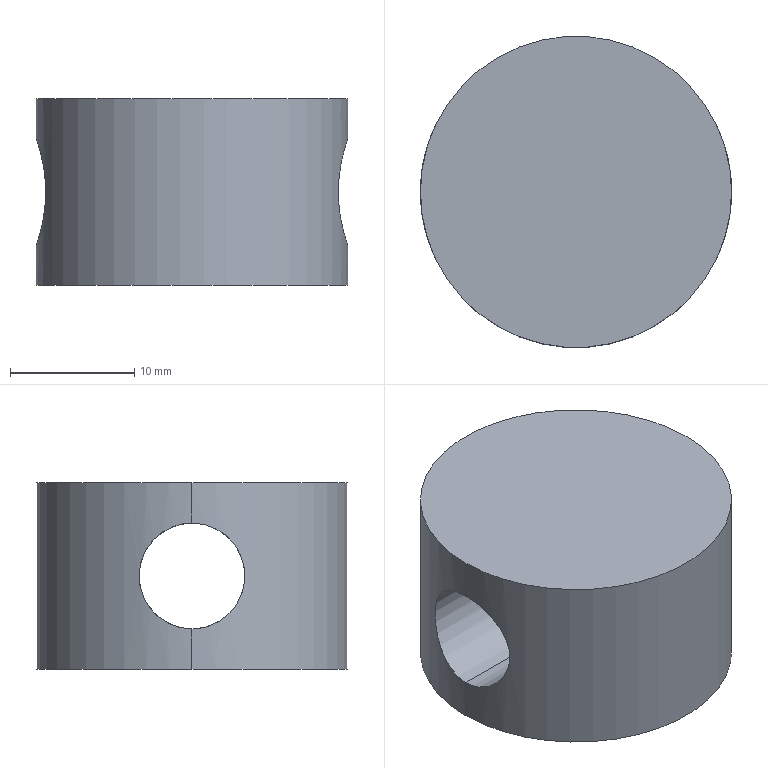Part | STEP file | Nylon shaft QY-1-30 | 1 solid | 6 faces | box 25 x 25 x 15 mm | volume 5965 mm3 | cylinder 4 | plane 2 | commonest cylinder face diameters 8.5 x2 25 x2
STEP:
#1=CARTESIAN_POINT('',(0.,0.,0.));
#2=DIRECTION('',(0.,0.,1.));
#3=DIRECTION('',(1.,0.,0.));
#4=AXIS2_PLACEMENT_3D('',#1,#2,#3);
#5=CARTESIAN_POINT('',(12.5,0.,11.75));
#6=VERTEX_POINT('',#5);
#7=CARTESIAN_POINT('',(-12.5,0.,11.75));
#8=VERTEX_POINT('',#7);
#9=CARTESIAN_POINT('',(0.,0.,11.75));
#10=DIRECTION('',(-1.,0.,0.));
#11=VECTOR('',#10,1.);
#12=LINE('',#9,#11);
#13=CARTESIAN_POINT('',(0.,0.,7.5));
#14=DIRECTION('',(-1.,0.,0.));
#15=DIRECTION('',(0.,0.,1.));
#16=AXIS2_PLACEMENT_3D('',#13,#14,#15);
#17=CYLINDRICAL_SURFACE('',#16,4.25);
#18=CARTESIAN_POINT('',(6.283,0.));
#19=DIRECTION('',(0.,1.));
#20=VECTOR('',#19,1.);
#21=LINE('',#18,#20);
#22=(GEOMETRIC_REPRESENTATION_CONTEXT(2)PARAMETRIC_REPRESENTATION_CONTEXT()REPRESENTATION_CONTEXT('',''));
#23=DEFINITIONAL_REPRESENTATION('',(#21),#22);
#24=PCURVE('',#17,#23);
#25=CARTESIAN_POINT('',(0.,0.,7.5));
#26=DIRECTION('',(-1.,0.,0.));
#27=DIRECTION('',(0.,0.,1.));
#28=AXIS2_PLACEMENT_3D('',#25,#26,#27);
#29=CYLINDRICAL_SURFACE('',#28,4.25);
#30=CARTESIAN_POINT('',(0.,0.));
#31=DIRECTION('',(0.,1.));
#32=VECTOR('',#31,1.);
#33=LINE('',#30,#32);
#34=(GEOMETRIC_REPRESENTATION_CONTEXT(2)PARAMETRIC_REPRESENTATION_CONTEXT()REPRESENTATION_CONTEXT('',''));
#35=DEFINITIONAL_REPRESENTATION('',(#33),#34);
#36=PCURVE('',#29,#35);
#37=SURFACE_CURVE('',#12,(#24,#36),.PCURVE_S1.);
#38=EDGE_CURVE('',#6,#8,#37,.T.);
#39=ORIENTED_EDGE('',*,*,#38,.T.);
#40=CARTESIAN_POINT('',(-12.5,0.,3.25));
#41=VERTEX_POINT('',#40);
#42=CARTESIAN_POINT('',(-12.5,0.,11.75));
#43=CARTESIAN_POINT('',(-12.5,-0.2788,11.75));
#44=CARTESIAN_POINT('',(-12.491,-0.5597,11.722));
#45=CARTESIAN_POINT('',(-12.454,-1.111,11.612));
#46=CARTESIAN_POINT('',(-12.427,-1.377,11.53));
#47=CARTESIAN_POINT('',(-12.359,-1.89,11.317));
#48=CARTESIAN_POINT('',(-12.318,-2.138,11.183));
#49=CARTESIAN_POINT('',(-12.229,-2.597,10.876));
#50=CARTESIAN_POINT('',(-12.182,-2.81,10.701));
#51=CARTESIAN_POINT('',(-12.036,-3.398,10.112));
#52=CARTESIAN_POINT('',(-11.939,-3.709,9.648));
#53=CARTESIAN_POINT('',(-11.833,-4.031,8.874));
#54=CARTESIAN_POINT('',(-11.804,-4.112,8.609));
#55=CARTESIAN_POINT('',(-11.766,-4.222,8.063));
#56=CARTESIAN_POINT('',(-11.755,-4.25,7.779));
#57=CARTESIAN_POINT('',(-11.755,-4.25,7.219));
#58=CARTESIAN_POINT('',(-11.765,-4.222,6.942));
#59=CARTESIAN_POINT('',(-11.804,-4.113,6.392));
#60=CARTESIAN_POINT('',(-11.833,-4.03,6.122));
#61=CARTESIAN_POINT('',(-11.904,-3.817,5.61));
#62=CARTESIAN_POINT('',(-11.946,-3.685,5.364));
#63=CARTESIAN_POINT('',(-12.037,-3.375,4.902));
#64=CARTESIAN_POINT('',(-12.085,-3.2,4.69));
#65=CARTESIAN_POINT('',(-12.182,-2.811,4.3));
#66=CARTESIAN_POINT('',(-12.23,-2.594,4.122));
#67=CARTESIAN_POINT('',(-12.319,-2.135,3.815));
#68=CARTESIAN_POINT('',(-12.359,-1.892,3.684));
#69=CARTESIAN_POINT('',(-12.427,-1.378,3.47));
#70=CARTESIAN_POINT('',(-12.454,-1.107,3.387));
#71=CARTESIAN_POINT('',(-12.49,-0.561,3.278));
#72=CARTESIAN_POINT('',(-12.5,-0.283,3.25));
#73=CARTESIAN_POINT('',(-12.5,0.,3.25));
#74=B_SPLINE_CURVE_WITH_KNOTS('',3,(#42,#43,#44,#45,#46,#47,#48,#49,#50,#51,#52,#53,#54,#55,#56,#57,#58,#59,#60,#61,#62,#63,#64,#65,#66,#67,#68,#69,#70,#71,#72,#73),.UNSPECIFIED.,.F.,.F.,(4,2,2,2,2,2,2,2,2,2,2,2,2,2,2,4),(0.01339,0.01422,0.01506,0.0159,0.01673,0.01841,0.01924,0.02008,0.02092,0.02175,0.02259,0.02343,0.02426,0.0251,0.02594,0.02677),.UNSPECIFIED.);
#75=CARTESIAN_POINT('',(6.283,12.5));
#76=CARTESIAN_POINT('',(6.267,12.5));
#77=CARTESIAN_POINT('',(6.235,12.499));
#78=CARTESIAN_POINT('',(6.187,12.494));
#79=CARTESIAN_POINT('',(6.139,12.486));
#80=CARTESIAN_POINT('',(6.091,12.474));
#81=CARTESIAN_POINT('',(6.043,12.46));
#82=CARTESIAN_POINT('',(5.996,12.442));
#83=CARTESIAN_POINT('',(5.948,12.422));
#84=CARTESIAN_POINT('',(5.901,12.399));
#85=CARTESIAN_POINT('',(5.853,12.374));
#86=CARTESIAN_POINT('',(5.805,12.347));
#87=CARTESIAN_POINT('',(5.758,12.317));
#88=CARTESIAN_POINT('',(5.71,12.286));
#89=CARTESIAN_POINT('',(5.663,12.254));
#90=CARTESIAN_POINT('',(5.616,12.22));
#91=CARTESIAN_POINT('',(5.569,12.186));
#92=CARTESIAN_POINT('',(5.521,12.151));
#93=CARTESIAN_POINT('',(5.474,12.115));
#94=CARTESIAN_POINT('',(5.426,12.08));
#95=CARTESIAN_POINT('',(5.379,12.045));
#96=CARTESIAN_POINT('',(5.332,12.011));
#97=CARTESIAN_POINT('',(5.285,11.978));
#98=CARTESIAN_POINT('',(5.237,11.947));
#99=CARTESIAN_POINT('',(5.19,11.916));
#100=CARTESIAN_POINT('',(5.142,11.888));
#101=CARTESIAN_POINT('',(5.095,11.861));
#102=CARTESIAN_POINT('',(5.047,11.837));
#103=CARTESIAN_POINT('',(4.999,11.816));
#104=CARTESIAN_POINT('',(4.952,11.798));
#105=CARTESIAN_POINT('',(4.904,11.783));
#106=CARTESIAN_POINT('',(4.857,11.771));
#107=CARTESIAN_POINT('',(4.808,11.762));
#108=CARTESIAN_POINT('',(4.76,11.757));
#109=CARTESIAN_POINT('',(4.712,11.755));
#110=CARTESIAN_POINT('',(4.664,11.757));
#111=CARTESIAN_POINT('',(4.617,11.762));
#112=CARTESIAN_POINT('',(4.569,11.77));
#113=CARTESIAN_POINT('',(4.521,11.782));
#114=CARTESIAN_POINT('',(4.473,11.798));
#115=CARTESIAN_POINT('',(4.425,11.816));
#116=CARTESIAN_POINT('',(4.377,11.838));
#117=CARTESIAN_POINT('',(4.33,11.862));
#118=CARTESIAN_POINT('',(4.282,11.888));
#119=CARTESIAN_POINT('',(4.235,11.916));
#120=CARTESIAN_POINT('',(4.187,11.947));
#121=CARTESIAN_POINT('',(4.14,11.979));
#122=CARTESIAN_POINT('',(4.092,12.012));
#123=CARTESIAN_POINT('',(4.045,12.046));
#124=CARTESIAN_POINT('',(3.998,12.081));
#125=CARTESIAN_POINT('',(3.951,12.116));
#126=CARTESIAN_POINT('',(3.904,12.151));
#127=CARTESIAN_POINT('',(3.856,12.186));
#128=CARTESIAN_POINT('',(3.809,12.221));
#129=CARTESIAN_POINT('',(3.761,12.254));
#130=CARTESIAN_POINT('',(3.714,12.287));
#131=CARTESIAN_POINT('',(3.667,12.317));
#132=CARTESIAN_POINT('',(3.619,12.347));
#133=CARTESIAN_POINT('',(3.572,12.374));
#134=CARTESIAN_POINT('',(3.525,12.399));
#135=CARTESIAN_POINT('',(3.477,12.422));
#136=CARTESIAN_POINT('',(3.429,12.442));
#137=CARTESIAN_POINT('',(3.381,12.46));
#138=CARTESIAN_POINT('',(3.333,12.474));
#139=CARTESIAN_POINT('',(3.286,12.486));
#140=CARTESIAN_POINT('',(3.238,12.494));
#141=CARTESIAN_POINT('',(3.19,12.499));
#142=CARTESIAN_POINT('',(3.158,12.5));
#143=CARTESIAN_POINT('',(3.142,12.5));
#144=B_SPLINE_CURVE_WITH_KNOTS('',3,(#75,#76,#77,#78,#79,#80,#81,#82,#83,#84,#85,#86,#87,#88,#89,#90,#91,#92,#93,#94,#95,#96,#97,#98,#99,#100,#101,#102,#103,#104,#105,#106,#107,#108,#109,#110,#111,#112,#113,#114,#115,#116,#117,#118,#119,#120,#121,#122,#123,#124,#125,#126,#127,#128,#129,#130,#131,#132,#133,#134,#135,#136,#137,#138,#139,#140,#141,#142,#143),.UNSPECIFIED.,.F.,.F.,(4,1,1,1,1,1,1,1,1,1,1,1,1,1,1,1,1,1,1,1,1,1,1,1,1,1,1,1,1,1,1,1,1,1,1,1,1,1,1,1,1,1,1,1,1,1,1,1,1,1,1,1,1,1,1,1,1,1,1,1,1,1,1,1,1,1,4),(0.01339,0.01359,0.01379,0.014,0.0142,0.0144,0.0146,0.01481,0.01501,0.01521,0.01542,0.01562,0.01582,0.01602,0.01623,0.01643,0.01663,0.01684,0.01704,0.01724,0.01744,0.01765,0.01785,0.01805,0.01826,0.01846,0.01866,0.01886,0.01907,0.01927,0.01947,0.01967,0.01988,0.02008,0.02028,0.02049,0.02069,0.02089,0.02109,0.0213,0.0215,0.0217,0.02191,0.02211,0.02231,0.02251,0.02272,0.02292,0.02312,0.02333,0.02353,0.02373,0.02393,0.02414,0.02434,0.02454,0.02474,0.02495,0.02515,0.02535,0.02556,0.02576,0.02596,0.02616,0.02637,0.02657,0.02677),.QUASI_UNIFORM_KNOTS.);
#145=(GEOMETRIC_REPRESENTATION_CONTEXT(2)PARAMETRIC_REPRESENTATION_CONTEXT()REPRESENTATION_CONTEXT('',''));
#146=DEFINITIONAL_REPRESENTATION('',(#144),#145);
#147=PCURVE('',#17,#146);
#148=CARTESIAN_POINT('',(0.,0.,15.));
#149=DIRECTION('',(0.,0.,-1.));
#150=DIRECTION('',(-1.,0.,0.));
#151=AXIS2_PLACEMENT_3D('',#148,#149,#150);
#152=CYLINDRICAL_SURFACE('',#151,12.5);
#153=CARTESIAN_POINT('',(6.283,3.25));
#154=CARTESIAN_POINT('',(6.278,3.25));
#155=CARTESIAN_POINT('',(6.267,3.253));
#156=CARTESIAN_POINT('',(6.251,3.268));
#157=CARTESIAN_POINT('',(6.234,3.292));
#158=CARTESIAN_POINT('',(6.218,3.326));
#159=CARTESIAN_POINT('',(6.202,3.37));
#160=CARTESIAN_POINT('',(6.187,3.423));
#161=CARTESIAN_POINT('',(6.171,3.485));
#162=CARTESIAN_POINT('',(6.156,3.556));
#163=CARTESIAN_POINT('',(6.141,3.636));
#164=CARTESIAN_POINT('',(6.126,3.725));
#165=CARTESIAN_POINT('',(6.112,3.822));
#166=CARTESIAN_POINT('',(6.098,3.928));
#167=CARTESIAN_POINT('',(6.084,4.041));
#168=CARTESIAN_POINT('',(6.071,4.161));
#169=CARTESIAN_POINT('',(6.058,4.289));
#170=CARTESIAN_POINT('',(6.046,4.424));
#171=CARTESIAN_POINT('',(6.034,4.567));
#172=CARTESIAN_POINT('',(6.023,4.716));
#173=CARTESIAN_POINT('',(6.013,4.871));
#174=CARTESIAN_POINT('',(6.003,5.031));
#175=CARTESIAN_POINT('',(5.993,5.197));
#176=CARTESIAN_POINT('',(5.984,5.369));
#177=CARTESIAN_POINT('',(5.976,5.546));
#178=CARTESIAN_POINT('',(5.969,5.727));
#179=CARTESIAN_POINT('',(5.962,5.914));
#180=CARTESIAN_POINT('',(5.956,6.104));
#181=CARTESIAN_POINT('',(5.951,6.296));
#182=CARTESIAN_POINT('',(5.946,6.491));
#183=CARTESIAN_POINT('',(5.943,6.688));
#184=CARTESIAN_POINT('',(5.94,6.889));
#185=CARTESIAN_POINT('',(5.938,7.092));
#186=CARTESIAN_POINT('',(5.937,7.297));
#187=CARTESIAN_POINT('',(5.936,7.501));
#188=CARTESIAN_POINT('',(5.937,7.704));
#189=CARTESIAN_POINT('',(5.938,7.906));
#190=CARTESIAN_POINT('',(5.94,8.108));
#191=CARTESIAN_POINT('',(5.943,8.308));
#192=CARTESIAN_POINT('',(5.946,8.507));
#193=CARTESIAN_POINT('',(5.951,8.704));
#194=CARTESIAN_POINT('',(5.956,8.898));
#195=CARTESIAN_POINT('',(5.962,9.088));
#196=CARTESIAN_POINT('',(5.969,9.273));
#197=CARTESIAN_POINT('',(5.976,9.454));
#198=CARTESIAN_POINT('',(5.984,9.632));
#199=CARTESIAN_POINT('',(5.993,9.804));
#200=CARTESIAN_POINT('',(6.003,9.971));
#201=CARTESIAN_POINT('',(6.013,10.132));
#202=CARTESIAN_POINT('',(6.023,10.286));
#203=CARTESIAN_POINT('',(6.035,10.434));
#204=CARTESIAN_POINT('',(6.046,10.576));
#205=CARTESIAN_POINT('',(6.058,10.712));
#206=CARTESIAN_POINT('',(6.071,10.84));
#207=CARTESIAN_POINT('',(6.084,10.962));
#208=CARTESIAN_POINT('',(6.098,11.074));
#209=CARTESIAN_POINT('',(6.112,11.179));
#210=CARTESIAN_POINT('',(6.126,11.275));
#211=CARTESIAN_POINT('',(6.141,11.364));
#212=CARTESIAN_POINT('',(6.156,11.444));
#213=CARTESIAN_POINT('',(6.171,11.515));
#214=CARTESIAN_POINT('',(6.187,11.577));
#215=CARTESIAN_POINT('',(6.203,11.631));
#216=CARTESIAN_POINT('',(6.218,11.674));
#217=CARTESIAN_POINT('',(6.234,11.708));
#218=CARTESIAN_POINT('',(6.251,11.732));
#219=CARTESIAN_POINT('',(6.267,11.747));
#220=CARTESIAN_POINT('',(6.278,11.75));
#221=CARTESIAN_POINT('',(6.283,11.75));
#222=B_SPLINE_CURVE_WITH_KNOTS('',3,(#153,#154,#155,#156,#157,#158,#159,#160,#161,#162,#163,#164,#165,#166,#167,#168,#169,#170,#171,#172,#173,#174,#175,#176,#177,#178,#179,#180,#181,#182,#183,#184,#185,#186,#187,#188,#189,#190,#191,#192,#193,#194,#195,#196,#197,#198,#199,#200,#201,#202,#203,#204,#205,#206,#207,#208,#209,#210,#211,#212,#213,#214,#215,#216,#217,#218,#219,#220,#221),.UNSPECIFIED.,.F.,.F.,(4,1,1,1,1,1,1,1,1,1,1,1,1,1,1,1,1,1,1,1,1,1,1,1,1,1,1,1,1,1,1,1,1,1,1,1,1,1,1,1,1,1,1,1,1,1,1,1,1,1,1,1,1,1,1,1,1,1,1,1,1,1,1,1,1,1,4),(0.01339,0.01359,0.01379,0.014,0.0142,0.0144,0.0146,0.01481,0.01501,0.01521,0.01542,0.01562,0.01582,0.01602,0.01623,0.01643,0.01663,0.01684,0.01704,0.01724,0.01744,0.01765,0.01785,0.01805,0.01826,0.01846,0.01866,0.01886,0.01907,0.01927,0.01947,0.01967,0.01988,0.02008,0.02028,0.02049,0.02069,0.02089,0.02109,0.0213,0.0215,0.0217,0.02191,0.02211,0.02231,0.02251,0.02272,0.02292,0.02312,0.02333,0.02353,0.02373,0.02393,0.02414,0.02434,0.02454,0.02474,0.02495,0.02515,0.02535,0.02556,0.02576,0.02596,0.02616,0.02637,0.02657,0.02677),.QUASI_UNIFORM_KNOTS.);
#223=(GEOMETRIC_REPRESENTATION_CONTEXT(2)PARAMETRIC_REPRESENTATION_CONTEXT()REPRESENTATION_CONTEXT('',''));
#224=DEFINITIONAL_REPRESENTATION('',(#222),#223);
#225=PCURVE('',#152,#224);
#226=SURFACE_CURVE('',#74,(#147,#225),.PCURVE_S1.);
#227=EDGE_CURVE('',#8,#41,#226,.T.);
#228=ORIENTED_EDGE('',*,*,#227,.T.);
#229=CARTESIAN_POINT('',(12.5,0.,3.25));
#230=VERTEX_POINT('',#229);
#231=CARTESIAN_POINT('',(0.,0.,3.25));
#232=DIRECTION('',(-1.,0.,0.));
#233=VECTOR('',#232,1.);
#234=LINE('',#231,#233);
#235=CARTESIAN_POINT('',(3.142,0.));
#236=DIRECTION('',(0.,1.));
#237=VECTOR('',#236,1.);
#238=LINE('',#235,#237);
#239=(GEOMETRIC_REPRESENTATION_CONTEXT(2)PARAMETRIC_REPRESENTATION_CONTEXT()REPRESENTATION_CONTEXT('',''));
#240=DEFINITIONAL_REPRESENTATION('',(#238),#239);
#241=PCURVE('',#17,#240);
#242=CARTESIAN_POINT('',(3.142,0.));
#243=DIRECTION('',(0.,1.));
#244=VECTOR('',#243,1.);
#245=LINE('',#242,#244);
#246=(GEOMETRIC_REPRESENTATION_CONTEXT(2)PARAMETRIC_REPRESENTATION_CONTEXT()REPRESENTATION_CONTEXT('',''));
#247=DEFINITIONAL_REPRESENTATION('',(#245),#246);
#248=PCURVE('',#29,#247);
#249=SURFACE_CURVE('',#234,(#241,#248),.PCURVE_S1.);
#250=EDGE_CURVE('',#230,#41,#249,.T.);
#251=ORIENTED_EDGE('',*,*,#250,.F.);
#252=CARTESIAN_POINT('',(12.5,0.,3.25));
#253=CARTESIAN_POINT('',(12.5,-0.2788,3.25));
#254=CARTESIAN_POINT('',(12.491,-0.5597,3.278));
#255=CARTESIAN_POINT('',(12.454,-1.111,3.388));
#256=CARTESIAN_POINT('',(12.427,-1.377,3.47));
#257=CARTESIAN_POINT('',(12.359,-1.89,3.683));
#258=CARTESIAN_POINT('',(12.318,-2.138,3.817));
#259=CARTESIAN_POINT('',(12.229,-2.597,4.124));
#260=CARTESIAN_POINT('',(12.182,-2.81,4.299));
#261=CARTESIAN_POINT('',(12.036,-3.398,4.888));
#262=CARTESIAN_POINT('',(11.939,-3.709,5.352));
#263=CARTESIAN_POINT('',(11.833,-4.031,6.126));
#264=CARTESIAN_POINT('',(11.804,-4.112,6.391));
#265=CARTESIAN_POINT('',(11.766,-4.222,6.937));
#266=CARTESIAN_POINT('',(11.755,-4.25,7.221));
#267=CARTESIAN_POINT('',(11.755,-4.25,7.781));
#268=CARTESIAN_POINT('',(11.765,-4.222,8.058));
#269=CARTESIAN_POINT('',(11.804,-4.113,8.608));
#270=CARTESIAN_POINT('',(11.833,-4.03,8.878));
#271=CARTESIAN_POINT('',(11.904,-3.817,9.39));
#272=CARTESIAN_POINT('',(11.946,-3.685,9.636));
#273=CARTESIAN_POINT('',(12.037,-3.375,10.098));
#274=CARTESIAN_POINT('',(12.085,-3.2,10.31));
#275=CARTESIAN_POINT('',(12.182,-2.811,10.7));
#276=CARTESIAN_POINT('',(12.23,-2.594,10.878));
#277=CARTESIAN_POINT('',(12.319,-2.135,11.185));
#278=CARTESIAN_POINT('',(12.359,-1.892,11.316));
#279=CARTESIAN_POINT('',(12.427,-1.378,11.53));
#280=CARTESIAN_POINT('',(12.454,-1.107,11.613));
#281=CARTESIAN_POINT('',(12.49,-0.561,11.722));
#282=CARTESIAN_POINT('',(12.5,-0.283,11.75));
#283=CARTESIAN_POINT('',(12.5,0.,11.75));
#284=B_SPLINE_CURVE_WITH_KNOTS('',3,(#252,#253,#254,#255,#256,#257,#258,#259,#260,#261,#262,#263,#264,#265,#266,#267,#268,#269,#270,#271,#272,#273,#274,#275,#276,#277,#278,#279,#280,#281,#282,#283),.UNSPECIFIED.,.F.,.F.,(4,2,2,2,2,2,2,2,2,2,2,2,2,2,2,4),(0.01339,0.01422,0.01506,0.0159,0.01673,0.01841,0.01924,0.02008,0.02092,0.02175,0.02259,0.02343,0.02426,0.0251,0.02594,0.02677),.UNSPECIFIED.);
#285=CARTESIAN_POINT('',(3.142,-12.5));
#286=CARTESIAN_POINT('',(3.157,-12.5));
#287=CARTESIAN_POINT('',(3.189,-12.499));
#288=CARTESIAN_POINT('',(3.237,-12.494));
#289=CARTESIAN_POINT('',(3.285,-12.486));
#290=CARTESIAN_POINT('',(3.333,-12.474));
#291=CARTESIAN_POINT('',(3.381,-12.46));
#292=CARTESIAN_POINT('',(3.429,-12.442));
#293=CARTESIAN_POINT('',(3.477,-12.422));
#294=CARTESIAN_POINT('',(3.524,-12.399));
#295=CARTESIAN_POINT('',(3.572,-12.374));
#296=CARTESIAN_POINT('',(3.619,-12.347));
#297=CARTESIAN_POINT('',(3.667,-12.317));
#298=CARTESIAN_POINT('',(3.715,-12.286));
#299=CARTESIAN_POINT('',(3.762,-12.254));
#300=CARTESIAN_POINT('',(3.809,-12.22));
#301=CARTESIAN_POINT('',(3.856,-12.186));
#302=CARTESIAN_POINT('',(3.903,-12.151));
#303=CARTESIAN_POINT('',(3.951,-12.115));
#304=CARTESIAN_POINT('',(3.998,-12.08));
#305=CARTESIAN_POINT('',(4.046,-12.045));
#306=CARTESIAN_POINT('',(4.093,-12.011));
#307=CARTESIAN_POINT('',(4.14,-11.978));
#308=CARTESIAN_POINT('',(4.187,-11.947));
#309=CARTESIAN_POINT('',(4.235,-11.916));
#310=CARTESIAN_POINT('',(4.282,-11.888));
#311=CARTESIAN_POINT('',(4.33,-11.861));
#312=CARTESIAN_POINT('',(4.378,-11.837));
#313=CARTESIAN_POINT('',(4.425,-11.816));
#314=CARTESIAN_POINT('',(4.473,-11.798));
#315=CARTESIAN_POINT('',(4.52,-11.783));
#316=CARTESIAN_POINT('',(4.568,-11.771));
#317=CARTESIAN_POINT('',(4.616,-11.762));
#318=CARTESIAN_POINT('',(4.665,-11.757));
#319=CARTESIAN_POINT('',(4.713,-11.755));
#320=CARTESIAN_POINT('',(4.76,-11.757));
#321=CARTESIAN_POINT('',(4.808,-11.762));
#322=CARTESIAN_POINT('',(4.856,-11.77));
#323=CARTESIAN_POINT('',(4.904,-11.782));
#324=CARTESIAN_POINT('',(4.952,-11.798));
#325=CARTESIAN_POINT('',(5.,-11.816));
#326=CARTESIAN_POINT('',(5.047,-11.838));
#327=CARTESIAN_POINT('',(5.095,-11.862));
#328=CARTESIAN_POINT('',(5.143,-11.888));
#329=CARTESIAN_POINT('',(5.19,-11.916));
#330=CARTESIAN_POINT('',(5.238,-11.947));
#331=CARTESIAN_POINT('',(5.285,-11.979));
#332=CARTESIAN_POINT('',(5.333,-12.012));
#333=CARTESIAN_POINT('',(5.38,-12.046));
#334=CARTESIAN_POINT('',(5.427,-12.081));
#335=CARTESIAN_POINT('',(5.474,-12.116));
#336=CARTESIAN_POINT('',(5.521,-12.151));
#337=CARTESIAN_POINT('',(5.569,-12.186));
#338=CARTESIAN_POINT('',(5.616,-12.221));
#339=CARTESIAN_POINT('',(5.664,-12.254));
#340=CARTESIAN_POINT('',(5.711,-12.287));
#341=CARTESIAN_POINT('',(5.758,-12.317));
#342=CARTESIAN_POINT('',(5.805,-12.347));
#343=CARTESIAN_POINT('',(5.853,-12.374));
#344=CARTESIAN_POINT('',(5.9,-12.399));
#345=CARTESIAN_POINT('',(5.948,-12.422));
#346=CARTESIAN_POINT('',(5.996,-12.442));
#347=CARTESIAN_POINT('',(6.044,-12.46));
#348=CARTESIAN_POINT('',(6.092,-12.474));
#349=CARTESIAN_POINT('',(6.139,-12.486));
#350=CARTESIAN_POINT('',(6.187,-12.494));
#351=CARTESIAN_POINT('',(6.235,-12.499));
#352=CARTESIAN_POINT('',(6.267,-12.5));
#353=CARTESIAN_POINT('',(6.283,-12.5));
#354=B_SPLINE_CURVE_WITH_KNOTS('',3,(#285,#286,#287,#288,#289,#290,#291,#292,#293,#294,#295,#296,#297,#298,#299,#300,#301,#302,#303,#304,#305,#306,#307,#308,#309,#310,#311,#312,#313,#314,#315,#316,#317,#318,#319,#320,#321,#322,#323,#324,#325,#326,#327,#328,#329,#330,#331,#332,#333,#334,#335,#336,#337,#338,#339,#340,#341,#342,#343,#344,#345,#346,#347,#348,#349,#350,#351,#352,#353),.UNSPECIFIED.,.F.,.F.,(4,1,1,1,1,1,1,1,1,1,1,1,1,1,1,1,1,1,1,1,1,1,1,1,1,1,1,1,1,1,1,1,1,1,1,1,1,1,1,1,1,1,1,1,1,1,1,1,1,1,1,1,1,1,1,1,1,1,1,1,1,1,1,1,1,1,4),(0.01339,0.01359,0.01379,0.014,0.0142,0.0144,0.0146,0.01481,0.01501,0.01521,0.01542,0.01562,0.01582,0.01602,0.01623,0.01643,0.01663,0.01684,0.01704,0.01724,0.01744,0.01765,0.01785,0.01805,0.01826,0.01846,0.01866,0.01886,0.01907,0.01927,0.01947,0.01967,0.01988,0.02008,0.02028,0.02049,0.02069,0.02089,0.02109,0.0213,0.0215,0.0217,0.02191,0.02211,0.02231,0.02251,0.02272,0.02292,0.02312,0.02333,0.02353,0.02373,0.02393,0.02414,0.02434,0.02454,0.02474,0.02495,0.02515,0.02535,0.02556,0.02576,0.02596,0.02616,0.02637,0.02657,0.02677),.QUASI_UNIFORM_KNOTS.);
#355=(GEOMETRIC_REPRESENTATION_CONTEXT(2)PARAMETRIC_REPRESENTATION_CONTEXT()REPRESENTATION_CONTEXT('',''));
#356=DEFINITIONAL_REPRESENTATION('',(#354),#355);
#357=PCURVE('',#17,#356);
#358=CARTESIAN_POINT('',(3.142,11.75));
#359=CARTESIAN_POINT('',(3.147,11.75));
#360=CARTESIAN_POINT('',(3.158,11.747));
#361=CARTESIAN_POINT('',(3.174,11.732));
#362=CARTESIAN_POINT('',(3.19,11.708));
#363=CARTESIAN_POINT('',(3.206,11.674));
#364=CARTESIAN_POINT('',(3.222,11.63));
#365=CARTESIAN_POINT('',(3.238,11.577));
#366=CARTESIAN_POINT('',(3.254,11.515));
#367=CARTESIAN_POINT('',(3.269,11.444));
#368=CARTESIAN_POINT('',(3.284,11.364));
#369=CARTESIAN_POINT('',(3.299,11.275));
#370=CARTESIAN_POINT('',(3.313,11.178));
#371=CARTESIAN_POINT('',(3.327,11.072));
#372=CARTESIAN_POINT('',(3.341,10.959));
#373=CARTESIAN_POINT('',(3.354,10.839));
#374=CARTESIAN_POINT('',(3.366,10.711));
#375=CARTESIAN_POINT('',(3.379,10.576));
#376=CARTESIAN_POINT('',(3.39,10.433));
#377=CARTESIAN_POINT('',(3.402,10.284));
#378=CARTESIAN_POINT('',(3.412,10.129));
#379=CARTESIAN_POINT('',(3.422,9.969));
#380=CARTESIAN_POINT('',(3.432,9.803));
#381=CARTESIAN_POINT('',(3.44,9.631));
#382=CARTESIAN_POINT('',(3.448,9.454));
#383=CARTESIAN_POINT('',(3.456,9.273));
#384=CARTESIAN_POINT('',(3.463,9.086));
#385=CARTESIAN_POINT('',(3.469,8.896));
#386=CARTESIAN_POINT('',(3.474,8.704));
#387=CARTESIAN_POINT('',(3.478,8.509));
#388=CARTESIAN_POINT('',(3.482,8.312));
#389=CARTESIAN_POINT('',(3.485,8.111));
#390=CARTESIAN_POINT('',(3.487,7.908));
#391=CARTESIAN_POINT('',(3.488,7.703));
#392=CARTESIAN_POINT('',(3.489,7.499));
#393=CARTESIAN_POINT('',(3.488,7.296));
#394=CARTESIAN_POINT('',(3.487,7.094));
#395=CARTESIAN_POINT('',(3.485,6.892));
#396=CARTESIAN_POINT('',(3.482,6.692));
#397=CARTESIAN_POINT('',(3.478,6.493));
#398=CARTESIAN_POINT('',(3.474,6.296));
#399=CARTESIAN_POINT('',(3.469,6.102));
#400=CARTESIAN_POINT('',(3.463,5.912));
#401=CARTESIAN_POINT('',(3.456,5.727));
#402=CARTESIAN_POINT('',(3.448,5.546));
#403=CARTESIAN_POINT('',(3.44,5.368));
#404=CARTESIAN_POINT('',(3.431,5.196));
#405=CARTESIAN_POINT('',(3.422,5.029));
#406=CARTESIAN_POINT('',(3.412,4.868));
#407=CARTESIAN_POINT('',(3.401,4.714));
#408=CARTESIAN_POINT('',(3.39,4.566));
#409=CARTESIAN_POINT('',(3.379,4.424));
#410=CARTESIAN_POINT('',(3.366,4.288));
#411=CARTESIAN_POINT('',(3.354,4.16));
#412=CARTESIAN_POINT('',(3.34,4.038));
#413=CARTESIAN_POINT('',(3.327,3.926));
#414=CARTESIAN_POINT('',(3.313,3.821));
#415=CARTESIAN_POINT('',(3.299,3.725));
#416=CARTESIAN_POINT('',(3.284,3.636));
#417=CARTESIAN_POINT('',(3.269,3.556));
#418=CARTESIAN_POINT('',(3.254,3.485));
#419=CARTESIAN_POINT('',(3.238,3.423));
#420=CARTESIAN_POINT('',(3.222,3.369));
#421=CARTESIAN_POINT('',(3.206,3.326));
#422=CARTESIAN_POINT('',(3.19,3.292));
#423=CARTESIAN_POINT('',(3.174,3.268));
#424=CARTESIAN_POINT('',(3.158,3.253));
#425=CARTESIAN_POINT('',(3.147,3.25));
#426=CARTESIAN_POINT('',(3.142,3.25));
#427=B_SPLINE_CURVE_WITH_KNOTS('',3,(#358,#359,#360,#361,#362,#363,#364,#365,#366,#367,#368,#369,#370,#371,#372,#373,#374,#375,#376,#377,#378,#379,#380,#381,#382,#383,#384,#385,#386,#387,#388,#389,#390,#391,#392,#393,#394,#395,#396,#397,#398,#399,#400,#401,#402,#403,#404,#405,#406,#407,#408,#409,#410,#411,#412,#413,#414,#415,#416,#417,#418,#419,#420,#421,#422,#423,#424,#425,#426),.UNSPECIFIED.,.F.,.F.,(4,1,1,1,1,1,1,1,1,1,1,1,1,1,1,1,1,1,1,1,1,1,1,1,1,1,1,1,1,1,1,1,1,1,1,1,1,1,1,1,1,1,1,1,1,1,1,1,1,1,1,1,1,1,1,1,1,1,1,1,1,1,1,1,1,1,4),(0.01339,0.01359,0.01379,0.014,0.0142,0.0144,0.0146,0.01481,0.01501,0.01521,0.01542,0.01562,0.01582,0.01602,0.01623,0.01643,0.01663,0.01684,0.01704,0.01724,0.01744,0.01765,0.01785,0.01805,0.01826,0.01846,0.01866,0.01886,0.01907,0.01927,0.01947,0.01967,0.01988,0.02008,0.02028,0.02049,0.02069,0.02089,0.02109,0.0213,0.0215,0.0217,0.02191,0.02211,0.02231,0.02251,0.02272,0.02292,0.02312,0.02333,0.02353,0.02373,0.02393,0.02414,0.02434,0.02454,0.02474,0.02495,0.02515,0.02535,0.02556,0.02576,0.02596,0.02616,0.02637,0.02657,0.02677),.QUASI_UNIFORM_KNOTS.);
#428=(GEOMETRIC_REPRESENTATION_CONTEXT(2)PARAMETRIC_REPRESENTATION_CONTEXT()REPRESENTATION_CONTEXT('',''));
#429=DEFINITIONAL_REPRESENTATION('',(#427),#428);
#430=PCURVE('',#152,#429);
#431=SURFACE_CURVE('',#284,(#357,#430),.PCURVE_S1.);
#432=EDGE_CURVE('',#230,#6,#431,.T.);
#433=ORIENTED_EDGE('',*,*,#432,.T.);
#434=EDGE_LOOP('',(#39,#228,#251,#433));
#435=FACE_BOUND('',#434,.F.);
#436=ADVANCED_FACE('',(#435),#17,.F.);
#437=CARTESIAN_POINT('',(12.5,0.,15.));
#438=VERTEX_POINT('',#437);
#439=CARTESIAN_POINT('',(-12.5,0.,15.));
#440=VERTEX_POINT('',#439);
#441=CARTESIAN_POINT('',(0.,0.,15.));
#442=DIRECTION('',(0.,0.,1.));
#443=DIRECTION('',(1.,0.,0.));
#444=AXIS2_PLACEMENT_3D('',#441,#442,#443);
#445=CIRCLE('',#444,12.5);
#446=CARTESIAN_POINT('',(0.,0.,15.));
#447=DIRECTION('',(0.,0.,-1.));
#448=DIRECTION('',(-1.,0.,0.));
#449=AXIS2_PLACEMENT_3D('',#446,#447,#448);
#450=CYLINDRICAL_SURFACE('',#449,12.5);
#451=CARTESIAN_POINT('',(3.142,0.));
#452=DIRECTION('',(-1.,0.));
#453=VECTOR('',#452,1.);
#454=LINE('',#451,#453);
#455=(GEOMETRIC_REPRESENTATION_CONTEXT(2)PARAMETRIC_REPRESENTATION_CONTEXT()REPRESENTATION_CONTEXT('',''));
#456=DEFINITIONAL_REPRESENTATION('',(#454),#455);
#457=PCURVE('',#450,#456);
#458=CARTESIAN_POINT('',(0.,0.,15.));
#459=DIRECTION('',(0.,0.,1.));
#460=DIRECTION('',(1.,0.,0.));
#461=AXIS2_PLACEMENT_3D('',#458,#459,#460);
#462=PLANE('',#461);
#463=CARTESIAN_POINT('',(0.,0.));
#464=DIRECTION('',(1.,0.));
#465=AXIS2_PLACEMENT_2D('',#463,#464);
#466=CIRCLE('',#465,12.5);
#467=(GEOMETRIC_REPRESENTATION_CONTEXT(2)PARAMETRIC_REPRESENTATION_CONTEXT()REPRESENTATION_CONTEXT('',''));
#468=DEFINITIONAL_REPRESENTATION('',(#466),#467);
#469=PCURVE('',#462,#468);
#470=SURFACE_CURVE('',#445,(#457,#469),.PCURVE_S1.);
#471=EDGE_CURVE('',#438,#440,#470,.T.);
#472=ORIENTED_EDGE('',*,*,#471,.F.);
#473=CARTESIAN_POINT('',(12.5,0.,15.));
#474=DIRECTION('',(0.,0.,-1.));
#475=VECTOR('',#474,1.);
#476=LINE('',#473,#475);
#477=CARTESIAN_POINT('',(3.142,0.));
#478=DIRECTION('',(0.,1.));
#479=VECTOR('',#478,1.);
#480=LINE('',#477,#479);
#481=(GEOMETRIC_REPRESENTATION_CONTEXT(2)PARAMETRIC_REPRESENTATION_CONTEXT()REPRESENTATION_CONTEXT('',''));
#482=DEFINITIONAL_REPRESENTATION('',(#480),#481);
#483=PCURVE('',#450,#482);
#484=CARTESIAN_POINT('',(3.142,0.));
#485=DIRECTION('',(0.,1.));
#486=VECTOR('',#485,1.);
#487=LINE('',#484,#486);
#488=(GEOMETRIC_REPRESENTATION_CONTEXT(2)PARAMETRIC_REPRESENTATION_CONTEXT()REPRESENTATION_CONTEXT('',''));
#489=DEFINITIONAL_REPRESENTATION('',(#487),#488);
#490=PCURVE('',#152,#489);
#491=SURFACE_CURVE('',#476,(#483,#490),.PCURVE_S1.);
#492=EDGE_CURVE('',#438,#6,#491,.T.);
#493=ORIENTED_EDGE('',*,*,#492,.T.);
#494=CARTESIAN_POINT('',(12.5,0.,11.75));
#495=CARTESIAN_POINT('',(12.5,0.2831,11.75));
#496=CARTESIAN_POINT('',(12.49,0.561,11.722));
#497=CARTESIAN_POINT('',(12.454,1.107,11.613));
#498=CARTESIAN_POINT('',(12.426,1.378,11.53));
#499=CARTESIAN_POINT('',(12.359,1.892,11.316));
#500=CARTESIAN_POINT('',(12.318,2.136,11.185));
#501=CARTESIAN_POINT('',(12.23,2.596,10.876));
#502=CARTESIAN_POINT('',(12.181,2.812,10.698));
#503=CARTESIAN_POINT('',(12.085,3.201,10.309));
#504=CARTESIAN_POINT('',(12.037,3.376,10.097));
#505=CARTESIAN_POINT('',(11.945,3.687,9.633));
#506=CARTESIAN_POINT('',(11.903,3.817,9.389));
#507=CARTESIAN_POINT('',(11.833,4.03,8.879));
#508=CARTESIAN_POINT('',(11.804,4.112,8.609));
#509=CARTESIAN_POINT('',(11.765,4.222,8.059));
#510=CARTESIAN_POINT('',(11.755,4.25,7.782));
#511=CARTESIAN_POINT('',(11.755,4.25,7.223));
#512=CARTESIAN_POINT('',(11.766,4.222,6.939));
#513=CARTESIAN_POINT('',(11.804,4.112,6.392));
#514=CARTESIAN_POINT('',(11.833,4.031,6.126));
#515=CARTESIAN_POINT('',(11.904,3.816,5.608));
#516=CARTESIAN_POINT('',(11.946,3.684,5.364));
#517=CARTESIAN_POINT('',(12.036,3.377,4.905));
#518=CARTESIAN_POINT('',(12.085,3.2,4.689));
#519=CARTESIAN_POINT('',(12.182,2.808,4.298));
#520=CARTESIAN_POINT('',(12.23,2.596,4.124));
#521=CARTESIAN_POINT('',(12.318,2.137,3.816));
#522=CARTESIAN_POINT('',(12.359,1.888,3.682));
#523=CARTESIAN_POINT('',(12.427,1.376,3.47));
#524=CARTESIAN_POINT('',(12.454,1.111,3.388));
#525=CARTESIAN_POINT('',(12.49,0.5605,3.278));
#526=CARTESIAN_POINT('',(12.5,0.2789,3.25));
#527=CARTESIAN_POINT('',(12.5,0.,3.25));
#528=B_SPLINE_CURVE_WITH_KNOTS('',3,(#494,#495,#496,#497,#498,#499,#500,#501,#502,#503,#504,#505,#506,#507,#508,#509,#510,#511,#512,#513,#514,#515,#516,#517,#518,#519,#520,#521,#522,#523,#524,#525,#526,#527),.UNSPECIFIED.,.F.,.F.,(4,2,2,2,2,2,2,2,2,2,2,2,2,2,2,2,4),(0.,0.0008368,0.001674,0.00251,0.003347,0.004184,0.005021,0.005857,0.006694,0.007531,0.008368,0.009204,0.01004,0.01088,0.01171,0.01255,0.01339),.UNSPECIFIED.);
#529=CARTESIAN_POINT('',(3.142,3.25));
#530=CARTESIAN_POINT('',(3.136,3.25));
#531=CARTESIAN_POINT('',(3.125,3.253));
#532=CARTESIAN_POINT('',(3.109,3.268));
#533=CARTESIAN_POINT('',(3.093,3.292));
#534=CARTESIAN_POINT('',(3.077,3.326));
#535=CARTESIAN_POINT('',(3.061,3.37));
#536=CARTESIAN_POINT('',(3.045,3.423));
#537=CARTESIAN_POINT('',(3.029,3.485));
#538=CARTESIAN_POINT('',(3.014,3.557));
#539=CARTESIAN_POINT('',(2.999,3.637));
#540=CARTESIAN_POINT('',(2.984,3.725));
#541=CARTESIAN_POINT('',(2.97,3.822));
#542=CARTESIAN_POINT('',(2.956,3.926));
#543=CARTESIAN_POINT('',(2.943,4.04));
#544=CARTESIAN_POINT('',(2.929,4.161));
#545=CARTESIAN_POINT('',(2.917,4.29));
#546=CARTESIAN_POINT('',(2.904,4.425));
#547=CARTESIAN_POINT('',(2.893,4.567));
#548=CARTESIAN_POINT('',(2.882,4.715));
#549=CARTESIAN_POINT('',(2.871,4.869));
#550=CARTESIAN_POINT('',(2.861,5.03));
#551=CARTESIAN_POINT('',(2.852,5.198));
#552=CARTESIAN_POINT('',(2.843,5.37));
#553=CARTESIAN_POINT('',(2.835,5.547));
#554=CARTESIAN_POINT('',(2.827,5.727));
#555=CARTESIAN_POINT('',(2.821,5.912));
#556=CARTESIAN_POINT('',(2.815,6.101));
#557=CARTESIAN_POINT('',(2.809,6.295));
#558=CARTESIAN_POINT('',(2.805,6.492));
#559=CARTESIAN_POINT('',(2.801,6.691));
#560=CARTESIAN_POINT('',(2.798,6.892));
#561=CARTESIAN_POINT('',(2.796,7.093));
#562=CARTESIAN_POINT('',(2.795,7.295));
#563=CARTESIAN_POINT('',(2.795,7.498));
#564=CARTESIAN_POINT('',(2.795,7.702));
#565=CARTESIAN_POINT('',(2.796,7.906));
#566=CARTESIAN_POINT('',(2.798,8.11));
#567=CARTESIAN_POINT('',(2.801,8.311));
#568=CARTESIAN_POINT('',(2.805,8.508));
#569=CARTESIAN_POINT('',(2.809,8.704));
#570=CARTESIAN_POINT('',(2.815,8.896));
#571=CARTESIAN_POINT('',(2.821,9.086));
#572=CARTESIAN_POINT('',(2.827,9.274));
#573=CARTESIAN_POINT('',(2.835,9.455));
#574=CARTESIAN_POINT('',(2.843,9.632));
#575=CARTESIAN_POINT('',(2.852,9.804));
#576=CARTESIAN_POINT('',(2.861,9.97));
#577=CARTESIAN_POINT('',(2.871,10.131));
#578=CARTESIAN_POINT('',(2.882,10.286));
#579=CARTESIAN_POINT('',(2.893,10.436));
#580=CARTESIAN_POINT('',(2.905,10.578));
#581=CARTESIAN_POINT('',(2.917,10.712));
#582=CARTESIAN_POINT('',(2.93,10.84));
#583=CARTESIAN_POINT('',(2.943,10.96));
#584=CARTESIAN_POINT('',(2.956,11.073));
#585=CARTESIAN_POINT('',(2.97,11.178));
#586=CARTESIAN_POINT('',(2.985,11.276));
#587=CARTESIAN_POINT('',(2.999,11.365));
#588=CARTESIAN_POINT('',(3.014,11.445));
#589=CARTESIAN_POINT('',(3.03,11.515));
#590=CARTESIAN_POINT('',(3.045,11.577));
#591=CARTESIAN_POINT('',(3.061,11.63));
#592=CARTESIAN_POINT('',(3.077,11.674));
#593=CARTESIAN_POINT('',(3.093,11.708));
#594=CARTESIAN_POINT('',(3.109,11.732));
#595=CARTESIAN_POINT('',(3.125,11.747));
#596=CARTESIAN_POINT('',(3.136,11.75));
#597=CARTESIAN_POINT('',(3.142,11.75));
#598=B_SPLINE_CURVE_WITH_KNOTS('',3,(#529,#530,#531,#532,#533,#534,#535,#536,#537,#538,#539,#540,#541,#542,#543,#544,#545,#546,#547,#548,#549,#550,#551,#552,#553,#554,#555,#556,#557,#558,#559,#560,#561,#562,#563,#564,#565,#566,#567,#568,#569,#570,#571,#572,#573,#574,#575,#576,#577,#578,#579,#580,#581,#582,#583,#584,#585,#586,#587,#588,#589,#590,#591,#592,#593,#594,#595,#596,#597),.UNSPECIFIED.,.F.,.F.,(4,1,1,1,1,1,1,1,1,1,1,1,1,1,1,1,1,1,1,1,1,1,1,1,1,1,1,1,1,1,1,1,1,1,1,1,1,1,1,1,1,1,1,1,1,1,1,1,1,1,1,1,1,1,1,1,1,1,1,1,1,1,1,1,1,1,4),(0.,0.0002028,0.0004057,0.0006085,0.0008114,0.001014,0.001217,0.00142,0.001623,0.001826,0.002028,0.002231,0.002434,0.002637,0.00284,0.003043,0.003246,0.003448,0.003651,0.003854,0.004057,0.00426,0.004463,0.004666,0.004868,0.005071,0.005274,0.005477,0.00568,0.005883,0.006085,0.006288,0.006491,0.006694,0.006897,0.0071,0.007303,0.007505,0.007708,0.007911,0.008114,0.008317,0.00852,0.008722,0.008925,0.009128,0.009331,0.009534,0.009737,0.00994,0.01014,0.01035,0.01055,0.01075,0.01095,0.01116,0.01136,0.01156,0.01177,0.01197,0.01217,0.01237,0.01258,0.01278,0.01298,0.01319,0.01339),.QUASI_UNIFORM_KNOTS.);
#599=(GEOMETRIC_REPRESENTATION_CONTEXT(2)PARAMETRIC_REPRESENTATION_CONTEXT()REPRESENTATION_CONTEXT('',''));
#600=DEFINITIONAL_REPRESENTATION('',(#598),#599);
#601=PCURVE('',#450,#600);
#602=CARTESIAN_POINT('',(0.,-12.5));
#603=CARTESIAN_POINT('',(0.01615,-12.5));
#604=CARTESIAN_POINT('',(0.0483,-12.499));
#605=CARTESIAN_POINT('',(0.09622,-12.494));
#606=CARTESIAN_POINT('',(0.1439,-12.486));
#607=CARTESIAN_POINT('',(0.1916,-12.474));
#608=CARTESIAN_POINT('',(0.2393,-12.46));
#609=CARTESIAN_POINT('',(0.2873,-12.442));
#610=CARTESIAN_POINT('',(0.3352,-12.422));
#611=CARTESIAN_POINT('',(0.3831,-12.399));
#612=CARTESIAN_POINT('',(0.4306,-12.374));
#613=CARTESIAN_POINT('',(0.478,-12.346));
#614=CARTESIAN_POINT('',(0.5253,-12.317));
#615=CARTESIAN_POINT('',(0.5726,-12.286));
#616=CARTESIAN_POINT('',(0.62,-12.254));
#617=CARTESIAN_POINT('',(0.6675,-12.22));
#618=CARTESIAN_POINT('',(0.715,-12.186));
#619=CARTESIAN_POINT('',(0.7623,-12.151));
#620=CARTESIAN_POINT('',(0.8094,-12.116));
#621=CARTESIAN_POINT('',(0.8564,-12.081));
#622=CARTESIAN_POINT('',(0.9036,-12.046));
#623=CARTESIAN_POINT('',(0.9509,-12.012));
#624=CARTESIAN_POINT('',(0.9987,-11.978));
#625=CARTESIAN_POINT('',(1.046,-11.946));
#626=CARTESIAN_POINT('',(1.094,-11.916));
#627=CARTESIAN_POINT('',(1.141,-11.888));
#628=CARTESIAN_POINT('',(1.188,-11.862));
#629=CARTESIAN_POINT('',(1.236,-11.838));
#630=CARTESIAN_POINT('',(1.283,-11.816));
#631=CARTESIAN_POINT('',(1.331,-11.798));
#632=CARTESIAN_POINT('',(1.379,-11.783));
#633=CARTESIAN_POINT('',(1.427,-11.77));
#634=CARTESIAN_POINT('',(1.475,-11.762));
#635=CARTESIAN_POINT('',(1.523,-11.757));
#636=CARTESIAN_POINT('',(1.57,-11.755));
#637=CARTESIAN_POINT('',(1.618,-11.756));
#638=CARTESIAN_POINT('',(1.666,-11.762));
#639=CARTESIAN_POINT('',(1.715,-11.771));
#640=CARTESIAN_POINT('',(1.763,-11.783));
#641=CARTESIAN_POINT('',(1.81,-11.798));
#642=CARTESIAN_POINT('',(1.858,-11.816));
#643=CARTESIAN_POINT('',(1.905,-11.837));
#644=CARTESIAN_POINT('',(1.953,-11.861));
#645=CARTESIAN_POINT('',(2.001,-11.888));
#646=CARTESIAN_POINT('',(2.049,-11.916));
#647=CARTESIAN_POINT('',(2.096,-11.947));
#648=CARTESIAN_POINT('',(2.143,-11.979));
#649=CARTESIAN_POINT('',(2.191,-12.012));
#650=CARTESIAN_POINT('',(2.238,-12.046));
#651=CARTESIAN_POINT('',(2.285,-12.081));
#652=CARTESIAN_POINT('',(2.333,-12.116));
#653=CARTESIAN_POINT('',(2.38,-12.151));
#654=CARTESIAN_POINT('',(2.427,-12.186));
#655=CARTESIAN_POINT('',(2.474,-12.22));
#656=CARTESIAN_POINT('',(2.521,-12.254));
#657=CARTESIAN_POINT('',(2.569,-12.286));
#658=CARTESIAN_POINT('',(2.616,-12.317));
#659=CARTESIAN_POINT('',(2.664,-12.347));
#660=CARTESIAN_POINT('',(2.712,-12.374));
#661=CARTESIAN_POINT('',(2.759,-12.399));
#662=CARTESIAN_POINT('',(2.807,-12.422));
#663=CARTESIAN_POINT('',(2.854,-12.442));
#664=CARTESIAN_POINT('',(2.902,-12.46));
#665=CARTESIAN_POINT('',(2.95,-12.474));
#666=CARTESIAN_POINT('',(2.998,-12.486));
#667=CARTESIAN_POINT('',(3.046,-12.494));
#668=CARTESIAN_POINT('',(3.094,-12.499));
#669=CARTESIAN_POINT('',(3.126,-12.5));
#670=CARTESIAN_POINT('',(3.142,-12.5));
#671=B_SPLINE_CURVE_WITH_KNOTS('',3,(#602,#603,#604,#605,#606,#607,#608,#609,#610,#611,#612,#613,#614,#615,#616,#617,#618,#619,#620,#621,#622,#623,#624,#625,#626,#627,#628,#629,#630,#631,#632,#633,#634,#635,#636,#637,#638,#639,#640,#641,#642,#643,#644,#645,#646,#647,#648,#649,#650,#651,#652,#653,#654,#655,#656,#657,#658,#659,#660,#661,#662,#663,#664,#665,#666,#667,#668,#669,#670),.UNSPECIFIED.,.F.,.F.,(4,1,1,1,1,1,1,1,1,1,1,1,1,1,1,1,1,1,1,1,1,1,1,1,1,1,1,1,1,1,1,1,1,1,1,1,1,1,1,1,1,1,1,1,1,1,1,1,1,1,1,1,1,1,1,1,1,1,1,1,1,1,1,1,1,1,4),(0.,0.0002028,0.0004057,0.0006085,0.0008114,0.001014,0.001217,0.00142,0.001623,0.001826,0.002028,0.002231,0.002434,0.002637,0.00284,0.003043,0.003246,0.003448,0.003651,0.003854,0.004057,0.00426,0.004463,0.004666,0.004868,0.005071,0.005274,0.005477,0.00568,0.005883,0.006085,0.006288,0.006491,0.006694,0.006897,0.0071,0.007303,0.007505,0.007708,0.007911,0.008114,0.008317,0.00852,0.008722,0.008925,0.009128,0.009331,0.009534,0.009737,0.00994,0.01014,0.01035,0.01055,0.01075,0.01095,0.01116,0.01136,0.01156,0.01177,0.01197,0.01217,0.01237,0.01258,0.01278,0.01298,0.01319,0.01339),.QUASI_UNIFORM_KNOTS.);
#672=(GEOMETRIC_REPRESENTATION_CONTEXT(2)PARAMETRIC_REPRESENTATION_CONTEXT()REPRESENTATION_CONTEXT('',''));
#673=DEFINITIONAL_REPRESENTATION('',(#671),#672);
#674=PCURVE('',#29,#673);
#675=SURFACE_CURVE('',#528,(#601,#674),.PCURVE_S1.);
#676=EDGE_CURVE('',#6,#230,#675,.T.);
#677=ORIENTED_EDGE('',*,*,#676,.T.);
#678=CARTESIAN_POINT('',(12.5,0.,0.));
#679=VERTEX_POINT('',#678);
#680=CARTESIAN_POINT('',(12.5,0.,15.));
#681=DIRECTION('',(0.,0.,-1.));
#682=VECTOR('',#681,1.);
#683=LINE('',#680,#682);
#684=CARTESIAN_POINT('',(3.142,0.));
#685=DIRECTION('',(0.,1.));
#686=VECTOR('',#685,1.);
#687=LINE('',#684,#686);
#688=(GEOMETRIC_REPRESENTATION_CONTEXT(2)PARAMETRIC_REPRESENTATION_CONTEXT()REPRESENTATION_CONTEXT('',''));
#689=DEFINITIONAL_REPRESENTATION('',(#687),#688);
#690=PCURVE('',#450,#689);
#691=CARTESIAN_POINT('',(3.142,0.));
#692=DIRECTION('',(0.,1.));
#693=VECTOR('',#692,1.);
#694=LINE('',#691,#693);
#695=(GEOMETRIC_REPRESENTATION_CONTEXT(2)PARAMETRIC_REPRESENTATION_CONTEXT()REPRESENTATION_CONTEXT('',''));
#696=DEFINITIONAL_REPRESENTATION('',(#694),#695);
#697=PCURVE('',#152,#696);
#698=SURFACE_CURVE('',#683,(#690,#697),.PCURVE_S1.);
#699=EDGE_CURVE('',#230,#679,#698,.T.);
#700=ORIENTED_EDGE('',*,*,#699,.T.);
#701=CARTESIAN_POINT('',(-12.5,0.,0.));
#702=VERTEX_POINT('',#701);
#703=CARTESIAN_POINT('',(0.,0.,0.));
#704=DIRECTION('',(0.,0.,1.));
#705=DIRECTION('',(1.,0.,0.));
#706=AXIS2_PLACEMENT_3D('',#703,#704,#705);
#707=CIRCLE('',#706,12.5);
#708=CARTESIAN_POINT('',(3.142,15.));
#709=DIRECTION('',(-1.,0.));
#710=VECTOR('',#709,1.);
#711=LINE('',#708,#710);
#712=(GEOMETRIC_REPRESENTATION_CONTEXT(2)PARAMETRIC_REPRESENTATION_CONTEXT()REPRESENTATION_CONTEXT('',''));
#713=DEFINITIONAL_REPRESENTATION('',(#711),#712);
#714=PCURVE('',#450,#713);
#715=CARTESIAN_POINT('',(0.,0.,0.));
#716=DIRECTION('',(0.,0.,1.));
#717=DIRECTION('',(1.,0.,0.));
#718=AXIS2_PLACEMENT_3D('',#715,#716,#717);
#719=PLANE('',#718);
#720=CARTESIAN_POINT('',(0.,0.));
#721=DIRECTION('',(1.,0.));
#722=AXIS2_PLACEMENT_2D('',#720,#721);
#723=CIRCLE('',#722,12.5);
#724=(GEOMETRIC_REPRESENTATION_CONTEXT(2)PARAMETRIC_REPRESENTATION_CONTEXT()REPRESENTATION_CONTEXT('',''));
#725=DEFINITIONAL_REPRESENTATION('',(#723),#724);
#726=PCURVE('',#719,#725);
#727=SURFACE_CURVE('',#707,(#714,#726),.PCURVE_S1.);
#728=EDGE_CURVE('',#679,#702,#727,.T.);
#729=ORIENTED_EDGE('',*,*,#728,.T.);
#730=CARTESIAN_POINT('',(-12.5,0.,15.));
#731=DIRECTION('',(0.,0.,-1.));
#732=VECTOR('',#731,1.);
#733=LINE('',#730,#732);
#734=CARTESIAN_POINT('',(0.,0.));
#735=DIRECTION('',(0.,1.));
#736=VECTOR('',#735,1.);
#737=LINE('',#734,#736);
#738=(GEOMETRIC_REPRESENTATION_CONTEXT(2)PARAMETRIC_REPRESENTATION_CONTEXT()REPRESENTATION_CONTEXT('',''));
#739=DEFINITIONAL_REPRESENTATION('',(#737),#738);
#740=PCURVE('',#450,#739);
#741=CARTESIAN_POINT('',(6.283,0.));
#742=DIRECTION('',(0.,1.));
#743=VECTOR('',#742,1.);
#744=LINE('',#741,#743);
#745=(GEOMETRIC_REPRESENTATION_CONTEXT(2)PARAMETRIC_REPRESENTATION_CONTEXT()REPRESENTATION_CONTEXT('',''));
#746=DEFINITIONAL_REPRESENTATION('',(#744),#745);
#747=PCURVE('',#152,#746);
#748=SURFACE_CURVE('',#733,(#740,#747),.PCURVE_S1.);
#749=EDGE_CURVE('',#41,#702,#748,.T.);
#750=ORIENTED_EDGE('',*,*,#749,.F.);
#751=CARTESIAN_POINT('',(-12.5,0.,3.25));
#752=CARTESIAN_POINT('',(-12.5,0.2831,3.25));
#753=CARTESIAN_POINT('',(-12.49,0.561,3.278));
#754=CARTESIAN_POINT('',(-12.454,1.107,3.387));
#755=CARTESIAN_POINT('',(-12.426,1.378,3.47));
#756=CARTESIAN_POINT('',(-12.359,1.892,3.684));
#757=CARTESIAN_POINT('',(-12.318,2.136,3.815));
#758=CARTESIAN_POINT('',(-12.23,2.596,4.124));
#759=CARTESIAN_POINT('',(-12.181,2.812,4.302));
#760=CARTESIAN_POINT('',(-12.085,3.201,4.691));
#761=CARTESIAN_POINT('',(-12.037,3.376,4.903));
#762=CARTESIAN_POINT('',(-11.945,3.687,5.367));
#763=CARTESIAN_POINT('',(-11.903,3.817,5.611));
#764=CARTESIAN_POINT('',(-11.833,4.03,6.121));
#765=CARTESIAN_POINT('',(-11.804,4.112,6.391));
#766=CARTESIAN_POINT('',(-11.765,4.222,6.941));
#767=CARTESIAN_POINT('',(-11.755,4.25,7.218));
#768=CARTESIAN_POINT('',(-11.755,4.25,7.777));
#769=CARTESIAN_POINT('',(-11.766,4.222,8.061));
#770=CARTESIAN_POINT('',(-11.804,4.112,8.608));
#771=CARTESIAN_POINT('',(-11.833,4.031,8.874));
#772=CARTESIAN_POINT('',(-11.904,3.816,9.392));
#773=CARTESIAN_POINT('',(-11.946,3.684,9.636));
#774=CARTESIAN_POINT('',(-12.036,3.377,10.095));
#775=CARTESIAN_POINT('',(-12.085,3.2,10.311));
#776=CARTESIAN_POINT('',(-12.182,2.808,10.702));
#777=CARTESIAN_POINT('',(-12.23,2.596,10.876));
#778=CARTESIAN_POINT('',(-12.318,2.137,11.184));
#779=CARTESIAN_POINT('',(-12.359,1.888,11.318));
#780=CARTESIAN_POINT('',(-12.427,1.376,11.53));
#781=CARTESIAN_POINT('',(-12.454,1.111,11.612));
#782=CARTESIAN_POINT('',(-12.49,0.5605,11.722));
#783=CARTESIAN_POINT('',(-12.5,0.2789,11.75));
#784=CARTESIAN_POINT('',(-12.5,0.,11.75));
#785=B_SPLINE_CURVE_WITH_KNOTS('',3,(#751,#752,#753,#754,#755,#756,#757,#758,#759,#760,#761,#762,#763,#764,#765,#766,#767,#768,#769,#770,#771,#772,#773,#774,#775,#776,#777,#778,#779,#780,#781,#782,#783,#784),.UNSPECIFIED.,.F.,.F.,(4,2,2,2,2,2,2,2,2,2,2,2,2,2,2,2,4),(0.,0.0008368,0.001674,0.00251,0.003347,0.004184,0.005021,0.005857,0.006694,0.007531,0.008368,0.009204,0.01004,0.01088,0.01171,0.01255,0.01339),.UNSPECIFIED.);
#786=CARTESIAN_POINT('',(0.,11.75));
#787=CARTESIAN_POINT('',(0.00549,11.75));
#788=CARTESIAN_POINT('',(0.01642,11.747));
#789=CARTESIAN_POINT('',(0.03268,11.732));
#790=CARTESIAN_POINT('',(0.04881,11.708));
#791=CARTESIAN_POINT('',(0.0648,11.674));
#792=CARTESIAN_POINT('',(0.0807,11.63));
#793=CARTESIAN_POINT('',(0.09651,11.577));
#794=CARTESIAN_POINT('',(0.1121,11.515));
#795=CARTESIAN_POINT('',(0.1275,11.443));
#796=CARTESIAN_POINT('',(0.1425,11.363));
#797=CARTESIAN_POINT('',(0.1571,11.275));
#798=CARTESIAN_POINT('',(0.1714,11.178));
#799=CARTESIAN_POINT('',(0.1853,11.074));
#800=CARTESIAN_POINT('',(0.1989,10.96));
#801=CARTESIAN_POINT('',(0.2121,10.839));
#802=CARTESIAN_POINT('',(0.2249,10.71));
#803=CARTESIAN_POINT('',(0.2371,10.575));
#804=CARTESIAN_POINT('',(0.2488,10.433));
#805=CARTESIAN_POINT('',(0.2599,10.285));
#806=CARTESIAN_POINT('',(0.2705,10.131));
#807=CARTESIAN_POINT('',(0.2805,9.97));
#808=CARTESIAN_POINT('',(0.29,9.802));
#809=CARTESIAN_POINT('',(0.2988,9.63));
#810=CARTESIAN_POINT('',(0.3069,9.453));
#811=CARTESIAN_POINT('',(0.3143,9.273));
#812=CARTESIAN_POINT('',(0.321,9.088));
#813=CARTESIAN_POINT('',(0.327,8.899));
#814=CARTESIAN_POINT('',(0.3323,8.705));
#815=CARTESIAN_POINT('',(0.3368,8.508));
#816=CARTESIAN_POINT('',(0.3405,8.309));
#817=CARTESIAN_POINT('',(0.3433,8.108));
#818=CARTESIAN_POINT('',(0.3454,7.907));
#819=CARTESIAN_POINT('',(0.3466,7.705));
#820=CARTESIAN_POINT('',(0.3471,7.502));
#821=CARTESIAN_POINT('',(0.3466,7.298));
#822=CARTESIAN_POINT('',(0.3454,7.094));
#823=CARTESIAN_POINT('',(0.3433,6.89));
#824=CARTESIAN_POINT('',(0.3404,6.689));
#825=CARTESIAN_POINT('',(0.3368,6.492));
#826=CARTESIAN_POINT('',(0.3323,6.296));
#827=CARTESIAN_POINT('',(0.3271,6.104));
#828=CARTESIAN_POINT('',(0.321,5.914));
#829=CARTESIAN_POINT('',(0.3143,5.726));
#830=CARTESIAN_POINT('',(0.3068,5.545));
#831=CARTESIAN_POINT('',(0.2987,5.368));
#832=CARTESIAN_POINT('',(0.2899,5.196));
#833=CARTESIAN_POINT('',(0.2805,5.03));
#834=CARTESIAN_POINT('',(0.2705,4.869));
#835=CARTESIAN_POINT('',(0.2598,4.714));
#836=CARTESIAN_POINT('',(0.2486,4.564));
#837=CARTESIAN_POINT('',(0.2369,4.422));
#838=CARTESIAN_POINT('',(0.2247,4.288));
#839=CARTESIAN_POINT('',(0.212,4.16));
#840=CARTESIAN_POINT('',(0.199,4.04));
#841=CARTESIAN_POINT('',(0.1854,3.927));
#842=CARTESIAN_POINT('',(0.1714,3.822));
#843=CARTESIAN_POINT('',(0.157,3.724));
#844=CARTESIAN_POINT('',(0.1422,3.635));
#845=CARTESIAN_POINT('',(0.1272,3.555));
#846=CARTESIAN_POINT('',(0.112,3.485));
#847=CARTESIAN_POINT('',(0.0966,3.423));
#848=CARTESIAN_POINT('',(0.08091,3.37));
#849=CARTESIAN_POINT('',(0.06494,3.326));
#850=CARTESIAN_POINT('',(0.04878,3.292));
#851=CARTESIAN_POINT('',(0.03254,3.268));
#852=CARTESIAN_POINT('',(0.01625,3.253));
#853=CARTESIAN_POINT('',(0.005408,3.25));
#854=CARTESIAN_POINT('',(0.,3.25));
#855=B_SPLINE_CURVE_WITH_KNOTS('',3,(#786,#787,#788,#789,#790,#791,#792,#793,#794,#795,#796,#797,#798,#799,#800,#801,#802,#803,#804,#805,#806,#807,#808,#809,#810,#811,#812,#813,#814,#815,#816,#817,#818,#819,#820,#821,#822,#823,#824,#825,#826,#827,#828,#829,#830,#831,#832,#833,#834,#835,#836,#837,#838,#839,#840,#841,#842,#843,#844,#845,#846,#847,#848,#849,#850,#851,#852,#853,#854),.UNSPECIFIED.,.F.,.F.,(4,1,1,1,1,1,1,1,1,1,1,1,1,1,1,1,1,1,1,1,1,1,1,1,1,1,1,1,1,1,1,1,1,1,1,1,1,1,1,1,1,1,1,1,1,1,1,1,1,1,1,1,1,1,1,1,1,1,1,1,1,1,1,1,1,1,4),(0.,0.0002028,0.0004057,0.0006085,0.0008114,0.001014,0.001217,0.00142,0.001623,0.001826,0.002028,0.002231,0.002434,0.002637,0.00284,0.003043,0.003246,0.003448,0.003651,0.003854,0.004057,0.00426,0.004463,0.004666,0.004868,0.005071,0.005274,0.005477,0.00568,0.005883,0.006085,0.006288,0.006491,0.006694,0.006897,0.0071,0.007303,0.007505,0.007708,0.007911,0.008114,0.008317,0.00852,0.008722,0.008925,0.009128,0.009331,0.009534,0.009737,0.00994,0.01014,0.01035,0.01055,0.01075,0.01095,0.01116,0.01136,0.01156,0.01177,0.01197,0.01217,0.01237,0.01258,0.01278,0.01298,0.01319,0.01339),.QUASI_UNIFORM_KNOTS.);
#856=(GEOMETRIC_REPRESENTATION_CONTEXT(2)PARAMETRIC_REPRESENTATION_CONTEXT()REPRESENTATION_CONTEXT('',''));
#857=DEFINITIONAL_REPRESENTATION('',(#855),#856);
#858=PCURVE('',#450,#857);
#859=CARTESIAN_POINT('',(3.142,12.5));
#860=CARTESIAN_POINT('',(3.125,12.5));
#861=CARTESIAN_POINT('',(3.093,12.499));
#862=CARTESIAN_POINT('',(3.045,12.494));
#863=CARTESIAN_POINT('',(2.998,12.486));
#864=CARTESIAN_POINT('',(2.95,12.474));
#865=CARTESIAN_POINT('',(2.902,12.46));
#866=CARTESIAN_POINT('',(2.854,12.442));
#867=CARTESIAN_POINT('',(2.806,12.422));
#868=CARTESIAN_POINT('',(2.759,12.399));
#869=CARTESIAN_POINT('',(2.711,12.374));
#870=CARTESIAN_POINT('',(2.664,12.346));
#871=CARTESIAN_POINT('',(2.616,12.317));
#872=CARTESIAN_POINT('',(2.569,12.286));
#873=CARTESIAN_POINT('',(2.522,12.254));
#874=CARTESIAN_POINT('',(2.474,12.22));
#875=CARTESIAN_POINT('',(2.427,12.186));
#876=CARTESIAN_POINT('',(2.379,12.151));
#877=CARTESIAN_POINT('',(2.332,12.116));
#878=CARTESIAN_POINT('',(2.285,12.081));
#879=CARTESIAN_POINT('',(2.238,12.046));
#880=CARTESIAN_POINT('',(2.191,12.012));
#881=CARTESIAN_POINT('',(2.143,11.978));
#882=CARTESIAN_POINT('',(2.095,11.946));
#883=CARTESIAN_POINT('',(2.048,11.916));
#884=CARTESIAN_POINT('',(2.001,11.888));
#885=CARTESIAN_POINT('',(1.954,11.862));
#886=CARTESIAN_POINT('',(1.906,11.838));
#887=CARTESIAN_POINT('',(1.858,11.816));
#888=CARTESIAN_POINT('',(1.81,11.798));
#889=CARTESIAN_POINT('',(1.762,11.783));
#890=CARTESIAN_POINT('',(1.714,11.77));
#891=CARTESIAN_POINT('',(1.667,11.762));
#892=CARTESIAN_POINT('',(1.619,11.757));
#893=CARTESIAN_POINT('',(1.571,11.755));
#894=CARTESIAN_POINT('',(1.523,11.756));
#895=CARTESIAN_POINT('',(1.475,11.762));
#896=CARTESIAN_POINT('',(1.427,11.771));
#897=CARTESIAN_POINT('',(1.379,11.783));
#898=CARTESIAN_POINT('',(1.331,11.798));
#899=CARTESIAN_POINT('',(1.284,11.816));
#900=CARTESIAN_POINT('',(1.236,11.837));
#901=CARTESIAN_POINT('',(1.188,11.861));
#902=CARTESIAN_POINT('',(1.14,11.888));
#903=CARTESIAN_POINT('',(1.093,11.916));
#904=CARTESIAN_POINT('',(1.045,11.947));
#905=CARTESIAN_POINT('',(0.9982,11.979));
#906=CARTESIAN_POINT('',(0.951,12.012));
#907=CARTESIAN_POINT('',(0.9036,12.046));
#908=CARTESIAN_POINT('',(0.8561,12.081));
#909=CARTESIAN_POINT('',(0.8087,12.116));
#910=CARTESIAN_POINT('',(0.7614,12.151));
#911=CARTESIAN_POINT('',(0.7142,12.186));
#912=CARTESIAN_POINT('',(0.6672,12.22));
#913=CARTESIAN_POINT('',(0.6201,12.254));
#914=CARTESIAN_POINT('',(0.5728,12.286));
#915=CARTESIAN_POINT('',(0.5253,12.317));
#916=CARTESIAN_POINT('',(0.4775,12.347));
#917=CARTESIAN_POINT('',(0.4298,12.374));
#918=CARTESIAN_POINT('',(0.3823,12.399));
#919=CARTESIAN_POINT('',(0.335,12.422));
#920=CARTESIAN_POINT('',(0.2875,12.442));
#921=CARTESIAN_POINT('',(0.2399,12.46));
#922=CARTESIAN_POINT('',(0.192,12.474));
#923=CARTESIAN_POINT('',(0.1439,12.486));
#924=CARTESIAN_POINT('',(0.09579,12.494));
#925=CARTESIAN_POINT('',(0.0478,12.499));
#926=CARTESIAN_POINT('',(0.01591,12.5));
#927=CARTESIAN_POINT('',(0.,12.5));
#928=B_SPLINE_CURVE_WITH_KNOTS('',3,(#859,#860,#861,#862,#863,#864,#865,#866,#867,#868,#869,#870,#871,#872,#873,#874,#875,#876,#877,#878,#879,#880,#881,#882,#883,#884,#885,#886,#887,#888,#889,#890,#891,#892,#893,#894,#895,#896,#897,#898,#899,#900,#901,#902,#903,#904,#905,#906,#907,#908,#909,#910,#911,#912,#913,#914,#915,#916,#917,#918,#919,#920,#921,#922,#923,#924,#925,#926,#927),.UNSPECIFIED.,.F.,.F.,(4,1,1,1,1,1,1,1,1,1,1,1,1,1,1,1,1,1,1,1,1,1,1,1,1,1,1,1,1,1,1,1,1,1,1,1,1,1,1,1,1,1,1,1,1,1,1,1,1,1,1,1,1,1,1,1,1,1,1,1,1,1,1,1,1,1,4),(0.,0.0002028,0.0004057,0.0006085,0.0008114,0.001014,0.001217,0.00142,0.001623,0.001826,0.002028,0.002231,0.002434,0.002637,0.00284,0.003043,0.003246,0.003448,0.003651,0.003854,0.004057,0.00426,0.004463,0.004666,0.004868,0.005071,0.005274,0.005477,0.00568,0.005883,0.006085,0.006288,0.006491,0.006694,0.006897,0.0071,0.007303,0.007505,0.007708,0.007911,0.008114,0.008317,0.00852,0.008722,0.008925,0.009128,0.009331,0.009534,0.009737,0.00994,0.01014,0.01035,0.01055,0.01075,0.01095,0.01116,0.01136,0.01156,0.01177,0.01197,0.01217,0.01237,0.01258,0.01278,0.01298,0.01319,0.01339),.QUASI_UNIFORM_KNOTS.);
#929=(GEOMETRIC_REPRESENTATION_CONTEXT(2)PARAMETRIC_REPRESENTATION_CONTEXT()REPRESENTATION_CONTEXT('',''));
#930=DEFINITIONAL_REPRESENTATION('',(#928),#929);
#931=PCURVE('',#29,#930);
#932=SURFACE_CURVE('',#785,(#858,#931),.PCURVE_S1.);
#933=EDGE_CURVE('',#41,#8,#932,.T.);
#934=ORIENTED_EDGE('',*,*,#933,.T.);
#935=CARTESIAN_POINT('',(-12.5,0.,15.));
#936=DIRECTION('',(0.,0.,-1.));
#937=VECTOR('',#936,1.);
#938=LINE('',#935,#937);
#939=CARTESIAN_POINT('',(0.,0.));
#940=DIRECTION('',(0.,1.));
#941=VECTOR('',#940,1.);
#942=LINE('',#939,#941);
#943=(GEOMETRIC_REPRESENTATION_CONTEXT(2)PARAMETRIC_REPRESENTATION_CONTEXT()REPRESENTATION_CONTEXT('',''));
#944=DEFINITIONAL_REPRESENTATION('',(#942),#943);
#945=PCURVE('',#450,#944);
#946=CARTESIAN_POINT('',(6.283,0.));
#947=DIRECTION('',(0.,1.));
#948=VECTOR('',#947,1.);
#949=LINE('',#946,#948);
#950=(GEOMETRIC_REPRESENTATION_CONTEXT(2)PARAMETRIC_REPRESENTATION_CONTEXT()REPRESENTATION_CONTEXT('',''));
#951=DEFINITIONAL_REPRESENTATION('',(#949),#950);
#952=PCURVE('',#152,#951);
#953=SURFACE_CURVE('',#938,(#945,#952),.PCURVE_S1.);
#954=EDGE_CURVE('',#440,#8,#953,.T.);
#955=ORIENTED_EDGE('',*,*,#954,.F.);
#956=EDGE_LOOP('',(#472,#493,#677,#700,#729,#750,#934,#955));
#957=FACE_BOUND('',#956,.T.);
#958=ADVANCED_FACE('',(#957),#450,.T.);
#959=ORIENTED_EDGE('',*,*,#492,.F.);
#960=CARTESIAN_POINT('',(0.,0.,15.));
#961=DIRECTION('',(0.,0.,1.));
#962=DIRECTION('',(1.,0.,0.));
#963=AXIS2_PLACEMENT_3D('',#960,#961,#962);
#964=CIRCLE('',#963,12.5);
#965=CARTESIAN_POINT('',(9.425,0.));
#966=DIRECTION('',(-1.,0.));
#967=VECTOR('',#966,1.);
#968=LINE('',#965,#967);
#969=(GEOMETRIC_REPRESENTATION_CONTEXT(2)PARAMETRIC_REPRESENTATION_CONTEXT()REPRESENTATION_CONTEXT('',''));
#970=DEFINITIONAL_REPRESENTATION('',(#968),#969);
#971=PCURVE('',#152,#970);
#972=CARTESIAN_POINT('',(0.,0.));
#973=DIRECTION('',(1.,0.));
#974=AXIS2_PLACEMENT_2D('',#972,#973);
#975=CIRCLE('',#974,12.5);
#976=(GEOMETRIC_REPRESENTATION_CONTEXT(2)PARAMETRIC_REPRESENTATION_CONTEXT()REPRESENTATION_CONTEXT('',''));
#977=DEFINITIONAL_REPRESENTATION('',(#975),#976);
#978=PCURVE('',#462,#977);
#979=SURFACE_CURVE('',#964,(#971,#978),.PCURVE_S1.);
#980=EDGE_CURVE('',#440,#438,#979,.T.);
#981=ORIENTED_EDGE('',*,*,#980,.F.);
#982=ORIENTED_EDGE('',*,*,#954,.T.);
#983=ORIENTED_EDGE('',*,*,#227,.T.);
#984=ORIENTED_EDGE('',*,*,#749,.T.);
#985=CARTESIAN_POINT('',(0.,0.,0.));
#986=DIRECTION('',(0.,0.,1.));
#987=DIRECTION('',(1.,0.,0.));
#988=AXIS2_PLACEMENT_3D('',#985,#986,#987);
#989=CIRCLE('',#988,12.5);
#990=CARTESIAN_POINT('',(9.425,15.));
#991=DIRECTION('',(-1.,0.));
#992=VECTOR('',#991,1.);
#993=LINE('',#990,#992);
#994=(GEOMETRIC_REPRESENTATION_CONTEXT(2)PARAMETRIC_REPRESENTATION_CONTEXT()REPRESENTATION_CONTEXT('',''));
#995=DEFINITIONAL_REPRESENTATION('',(#993),#994);
#996=PCURVE('',#152,#995);
#997=CARTESIAN_POINT('',(0.,0.));
#998=DIRECTION('',(1.,0.));
#999=AXIS2_PLACEMENT_2D('',#997,#998);
#1000=CIRCLE('',#999,12.5);
#1001=(GEOMETRIC_REPRESENTATION_CONTEXT(2)PARAMETRIC_REPRESENTATION_CONTEXT()REPRESENTATION_CONTEXT('',''));
#1002=DEFINITIONAL_REPRESENTATION('',(#1000),#1001);
#1003=PCURVE('',#719,#1002);
#1004=SURFACE_CURVE('',#989,(#996,#1003),.PCURVE_S1.);
#1005=EDGE_CURVE('',#702,#679,#1004,.T.);
#1006=ORIENTED_EDGE('',*,*,#1005,.T.);
#1007=ORIENTED_EDGE('',*,*,#699,.F.);
#1008=ORIENTED_EDGE('',*,*,#432,.T.);
#1009=EDGE_LOOP('',(#959,#981,#982,#983,#984,#1006,#1007,#1008));
#1010=FACE_BOUND('',#1009,.T.);
#1011=ADVANCED_FACE('',(#1010),#152,.T.);
#1012=ORIENTED_EDGE('',*,*,#980,.T.);
#1013=ORIENTED_EDGE('',*,*,#471,.T.);
#1014=EDGE_LOOP('',(#1012,#1013));
#1015=FACE_BOUND('',#1014,.T.);
#1016=ADVANCED_FACE('',(#1015),#462,.T.);
#1017=ORIENTED_EDGE('',*,*,#1005,.F.);
#1018=ORIENTED_EDGE('',*,*,#728,.F.);
#1019=EDGE_LOOP('',(#1017,#1018));
#1020=FACE_BOUND('',#1019,.T.);
#1021=ADVANCED_FACE('',(#1020),#719,.F.);
#1022=ORIENTED_EDGE('',*,*,#933,.T.);
#1023=ORIENTED_EDGE('',*,*,#38,.F.);
#1024=ORIENTED_EDGE('',*,*,#676,.T.);
#1025=ORIENTED_EDGE('',*,*,#250,.T.);
#1026=EDGE_LOOP('',(#1022,#1023,#1024,#1025));
#1027=FACE_BOUND('',#1026,.F.);
#1028=ADVANCED_FACE('',(#1027),#29,.F.);
#1029=CLOSED_SHELL('',(#436,#958,#1011,#1016,#1021,#1028));
#1030=MANIFOLD_SOLID_BREP('',#1029);
#1031=(LENGTH_UNIT()NAMED_UNIT(*)SI_UNIT(.MILLI.,.METRE.));
#1032=UNCERTAINTY_MEASURE_WITH_UNIT(LENGTH_MEASURE(0.0001),#1031,'','');
#1033=(NAMED_UNIT(*)PLANE_ANGLE_UNIT()SI_UNIT($,.RADIAN.));
#1034=(NAMED_UNIT(*)SI_UNIT($,.STERADIAN.)SOLID_ANGLE_UNIT());
#1035=(GEOMETRIC_REPRESENTATION_CONTEXT(3)GLOBAL_UNCERTAINTY_ASSIGNED_CONTEXT((#1032))GLOBAL_UNIT_ASSIGNED_CONTEXT((#1031,#1033,#1034))REPRESENTATION_CONTEXT('',''));
#1036=ADVANCED_BREP_SHAPE_REPRESENTATION('',(#4,#1030),#1035);